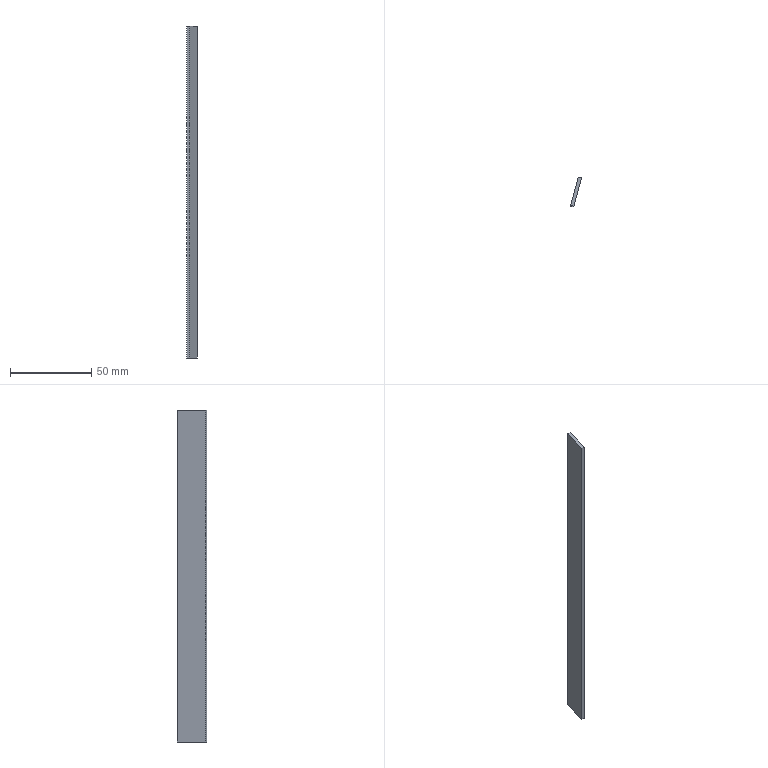Part | SolidWorks | features Extrusion 1 | 1 solid | 6 faces | box 6.591 x 17.904 x 204 mm | volume 7344 mm3 | plane 6
STEP:
#1=CARTESIAN_POINT('',(3213.188,1372.928,292.145));
#2=VERTEX_POINT('',#1);
#3=CARTESIAN_POINT('',(3213.188,1372.928,88.145));
#4=VERTEX_POINT('',#3);
#5=CARTESIAN_POINT('',(3213.188,1372.928,292.145));
#6=DIRECTION('',(0.,0.,-1.));
#7=VECTOR('',#6,1000.);
#8=LINE('',#5,#7);
#9=EDGE_CURVE('',#2,#4,#8,.T.);
#10=ORIENTED_EDGE('',*,*,#9,.F.);
#11=CARTESIAN_POINT('',(3215.119,1372.411,292.145));
#12=VERTEX_POINT('',#11);
#13=CARTESIAN_POINT('',(3215.119,1372.411,292.145));
#14=DIRECTION('',(-0.9659,0.2588,0.));
#15=VECTOR('',#14,1000.);
#16=LINE('',#13,#15);
#17=EDGE_CURVE('',#12,#2,#16,.T.);
#18=ORIENTED_EDGE('',*,*,#17,.F.);
#19=CARTESIAN_POINT('',(3215.119,1372.411,88.145));
#20=VERTEX_POINT('',#19);
#21=CARTESIAN_POINT('',(3215.119,1372.411,292.145));
#22=DIRECTION('',(0.,0.,-1.));
#23=VECTOR('',#22,1000.);
#24=LINE('',#21,#23);
#25=EDGE_CURVE('',#12,#20,#24,.T.);
#26=ORIENTED_EDGE('',*,*,#25,.T.);
#27=CARTESIAN_POINT('',(3215.119,1372.411,88.145));
#28=DIRECTION('',(-0.9659,0.2588,0.));
#29=VECTOR('',#28,1000.);
#30=LINE('',#27,#29);
#31=EDGE_CURVE('',#20,#4,#30,.T.);
#32=ORIENTED_EDGE('',*,*,#31,.T.);
#33=EDGE_LOOP('',(#10,#18,#26,#32));
#34=FACE_OUTER_BOUND('',#33,.T.);
#35=CARTESIAN_POINT('',(3215.119,1372.411,292.145));
#36=DIRECTION('',(0.2588,0.9659,0.));
#37=DIRECTION('',(-0.9659,0.2588,0.));
#38=AXIS2_PLACEMENT_3D('',#35,#36,#37);
#39=PLANE('',#38);
#40=ADVANCED_FACE('',(#34),#39,.T.);
#41=CARTESIAN_POINT('',(3208.529,1355.542,292.145));
#42=VERTEX_POINT('',#41);
#43=CARTESIAN_POINT('',(3208.529,1355.542,292.145));
#44=DIRECTION('',(0.2588,0.9659,0.));
#45=VECTOR('',#44,1000.);
#46=LINE('',#43,#45);
#47=EDGE_CURVE('',#42,#2,#46,.T.);
#48=ORIENTED_EDGE('',*,*,#47,.F.);
#49=CARTESIAN_POINT('',(3210.461,1355.024,292.145));
#50=VERTEX_POINT('',#49);
#51=CARTESIAN_POINT('',(3210.461,1355.024,292.145));
#52=DIRECTION('',(-0.9659,0.2588,0.));
#53=VECTOR('',#52,1000.);
#54=LINE('',#51,#53);
#55=EDGE_CURVE('',#50,#42,#54,.T.);
#56=ORIENTED_EDGE('',*,*,#55,.F.);
#57=CARTESIAN_POINT('',(3210.461,1355.024,292.145));
#58=DIRECTION('',(0.2588,0.9659,0.));
#59=VECTOR('',#58,1000.);
#60=LINE('',#57,#59);
#61=EDGE_CURVE('',#50,#12,#60,.T.);
#62=ORIENTED_EDGE('',*,*,#61,.T.);
#63=ORIENTED_EDGE('',*,*,#17,.T.);
#64=EDGE_LOOP('',(#48,#56,#62,#63));
#65=FACE_OUTER_BOUND('',#64,.T.);
#66=CARTESIAN_POINT('',(3210.461,1355.024,292.145));
#67=DIRECTION('',(0.,0.,1.));
#68=DIRECTION('',(0.,-1.,0.));
#69=AXIS2_PLACEMENT_3D('',#66,#67,#68);
#70=PLANE('',#69);
#71=ADVANCED_FACE('',(#65),#70,.T.);
#72=CARTESIAN_POINT('',(3208.529,1355.542,88.145));
#73=VERTEX_POINT('',#72);
#74=CARTESIAN_POINT('',(3208.529,1355.542,88.145));
#75=DIRECTION('',(0.,0.,1.));
#76=VECTOR('',#75,1000.);
#77=LINE('',#74,#76);
#78=EDGE_CURVE('',#73,#42,#77,.T.);
#79=ORIENTED_EDGE('',*,*,#78,.F.);
#80=CARTESIAN_POINT('',(3210.461,1355.024,88.145));
#81=VERTEX_POINT('',#80);
#82=CARTESIAN_POINT('',(3210.461,1355.024,88.145));
#83=DIRECTION('',(-0.9659,0.2588,0.));
#84=VECTOR('',#83,1000.);
#85=LINE('',#82,#84);
#86=EDGE_CURVE('',#81,#73,#85,.T.);
#87=ORIENTED_EDGE('',*,*,#86,.F.);
#88=CARTESIAN_POINT('',(3210.461,1355.024,88.145));
#89=DIRECTION('',(0.,0.,1.));
#90=VECTOR('',#89,1000.);
#91=LINE('',#88,#90);
#92=EDGE_CURVE('',#81,#50,#91,.T.);
#93=ORIENTED_EDGE('',*,*,#92,.T.);
#94=ORIENTED_EDGE('',*,*,#55,.T.);
#95=EDGE_LOOP('',(#79,#87,#93,#94));
#96=FACE_OUTER_BOUND('',#95,.T.);
#97=CARTESIAN_POINT('',(3210.461,1355.024,88.145));
#98=DIRECTION('',(-0.2588,-0.9659,0.));
#99=DIRECTION('',(0.9659,-0.2588,0.));
#100=AXIS2_PLACEMENT_3D('',#97,#98,#99);
#101=PLANE('',#100);
#102=ADVANCED_FACE('',(#96),#101,.T.);
#103=CARTESIAN_POINT('',(3213.188,1372.928,88.145));
#104=DIRECTION('',(-0.2588,-0.9659,0.));
#105=VECTOR('',#104,1000.);
#106=LINE('',#103,#105);
#107=EDGE_CURVE('',#4,#73,#106,.T.);
#108=ORIENTED_EDGE('',*,*,#107,.F.);
#109=ORIENTED_EDGE('',*,*,#31,.F.);
#110=CARTESIAN_POINT('',(3215.119,1372.411,88.145));
#111=DIRECTION('',(-0.2588,-0.9659,0.));
#112=VECTOR('',#111,1000.);
#113=LINE('',#110,#112);
#114=EDGE_CURVE('',#20,#81,#113,.T.);
#115=ORIENTED_EDGE('',*,*,#114,.T.);
#116=ORIENTED_EDGE('',*,*,#86,.T.);
#117=EDGE_LOOP('',(#108,#109,#115,#116));
#118=FACE_OUTER_BOUND('',#117,.T.);
#119=CARTESIAN_POINT('',(3215.119,1372.411,88.145));
#120=DIRECTION('',(0.,0.,-1.));
#121=DIRECTION('',(-1.,0.,0.));
#122=AXIS2_PLACEMENT_3D('',#119,#120,#121);
#123=PLANE('',#122);
#124=ADVANCED_FACE('',(#118),#123,.T.);
#125=ORIENTED_EDGE('',*,*,#25,.F.);
#126=ORIENTED_EDGE('',*,*,#61,.F.);
#127=ORIENTED_EDGE('',*,*,#92,.F.);
#128=ORIENTED_EDGE('',*,*,#114,.F.);
#129=EDGE_LOOP('',(#125,#126,#127,#128));
#130=FACE_OUTER_BOUND('',#129,.T.);
#131=CARTESIAN_POINT('',(2656.645,-711.846,0.));
#132=DIRECTION('',(-0.9659,0.2588,0.));
#133=DIRECTION('',(-0.2588,-0.9659,0.));
#134=AXIS2_PLACEMENT_3D('',#131,#132,#133);
#135=PLANE('',#134);
#136=ADVANCED_FACE('',(#130),#135,.F.);
#137=ORIENTED_EDGE('',*,*,#9,.T.);
#138=ORIENTED_EDGE('',*,*,#107,.T.);
#139=ORIENTED_EDGE('',*,*,#78,.T.);
#140=ORIENTED_EDGE('',*,*,#47,.T.);
#141=EDGE_LOOP('',(#137,#138,#139,#140));
#142=FACE_OUTER_BOUND('',#141,.T.);
#143=CARTESIAN_POINT('',(2654.713,-711.328,0.));
#144=DIRECTION('',(-0.9659,0.2588,0.));
#145=DIRECTION('',(-0.2588,-0.9659,0.));
#146=AXIS2_PLACEMENT_3D('',#143,#144,#145);
#147=PLANE('',#146);
#148=ADVANCED_FACE('',(#142),#147,.T.);
#149=CLOSED_SHELL('',(#40,#71,#102,#124,#136,#148));
#150=MANIFOLD_SOLID_BREP('',#149);
#151=CARTESIAN_POINT('',(0.,0.,0.));
#152=DIRECTION('',(0.,0.,1.));
#153=DIRECTION('',(1.,0.,0.));
#154=AXIS2_PLACEMENT_3D('',#151,#152,#153);
#155=(LENGTH_UNIT()NAMED_UNIT(*)SI_UNIT(.MILLI.,.METRE.));
#156=UNCERTAINTY_MEASURE_WITH_UNIT(LENGTH_MEASURE(0.00001),#155,'','');
#157=(NAMED_UNIT(*)PLANE_ANGLE_UNIT()SI_UNIT($,.RADIAN.));
#158=(NAMED_UNIT(*)SI_UNIT($,.STERADIAN.)SOLID_ANGLE_UNIT());
#159=(GEOMETRIC_REPRESENTATION_CONTEXT(3)GLOBAL_UNCERTAINTY_ASSIGNED_CONTEXT((#156))GLOBAL_UNIT_ASSIGNED_CONTEXT((#155,#157,#158))REPRESENTATION_CONTEXT('',''));
#160=ADVANCED_BREP_SHAPE_REPRESENTATION('',(#150,#154),#159);